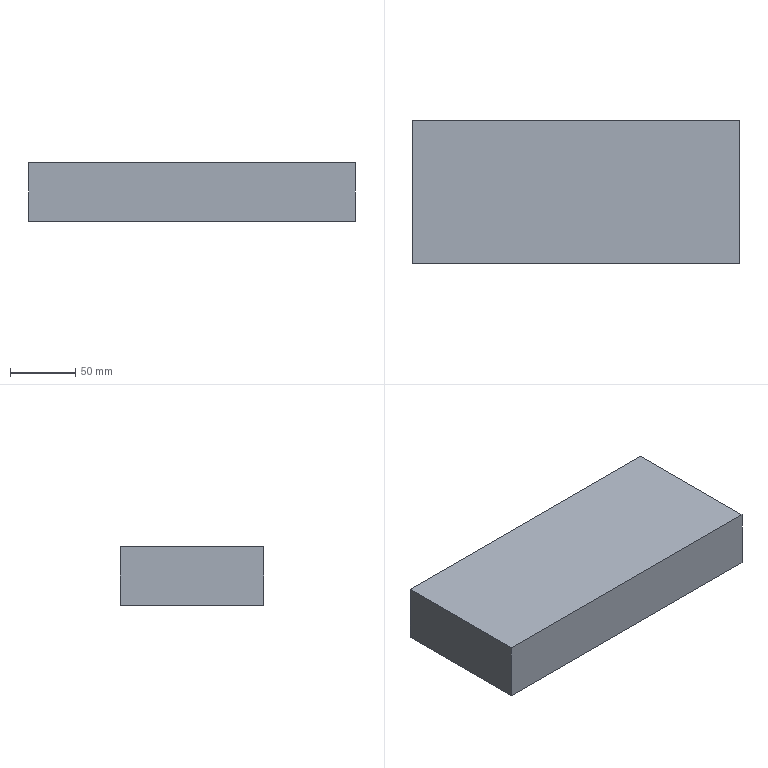Part | SolidWorks | features Extrusion 1 | 1 solid | 6 faces | box 250 x 110 x 45 mm | volume 1237500 mm3 | plane 6
STEP:
#1=CARTESIAN_POINT('',(-125.,55.,-22.5));
#2=VERTEX_POINT('',#1);
#3=CARTESIAN_POINT('',(-125.,-55.,-22.5));
#4=VERTEX_POINT('',#3);
#5=CARTESIAN_POINT('',(-125.,-55.,-22.5));
#6=DIRECTION('',(0.,-1.,0.));
#7=VECTOR('',#6,1000.);
#8=LINE('',#5,#7);
#9=EDGE_CURVE('',#2,#4,#8,.T.);
#10=ORIENTED_EDGE('',*,*,#9,.T.);
#11=CARTESIAN_POINT('',(-125.,-55.,22.5));
#12=VERTEX_POINT('',#11);
#13=CARTESIAN_POINT('',(-125.,-55.,22.5));
#14=DIRECTION('',(0.,0.,-1.));
#15=VECTOR('',#14,1000.);
#16=LINE('',#13,#15);
#17=EDGE_CURVE('',#12,#4,#16,.T.);
#18=ORIENTED_EDGE('',*,*,#17,.F.);
#19=CARTESIAN_POINT('',(-125.,55.,22.5));
#20=VERTEX_POINT('',#19);
#21=CARTESIAN_POINT('',(-125.,-55.,22.5));
#22=DIRECTION('',(0.,-1.,0.));
#23=VECTOR('',#22,1000.);
#24=LINE('',#21,#23);
#25=EDGE_CURVE('',#20,#12,#24,.T.);
#26=ORIENTED_EDGE('',*,*,#25,.F.);
#27=CARTESIAN_POINT('',(-125.,55.,22.5));
#28=DIRECTION('',(0.,0.,-1.));
#29=VECTOR('',#28,1000.);
#30=LINE('',#27,#29);
#31=EDGE_CURVE('',#20,#2,#30,.T.);
#32=ORIENTED_EDGE('',*,*,#31,.T.);
#33=EDGE_LOOP('',(#10,#18,#26,#32));
#34=FACE_OUTER_BOUND('',#33,.T.);
#35=CARTESIAN_POINT('',(-125.,-55.,22.5));
#36=DIRECTION('',(1.,0.,0.));
#37=DIRECTION('',(0.,0.,-1.));
#38=AXIS2_PLACEMENT_3D('',#35,#36,#37);
#39=PLANE('',#38);
#40=ADVANCED_FACE('',(#34),#39,.F.);
#41=CARTESIAN_POINT('',(125.,-55.,-22.5));
#42=VERTEX_POINT('',#41);
#43=CARTESIAN_POINT('',(125.,-55.,-22.5));
#44=DIRECTION('',(1.,0.,0.));
#45=VECTOR('',#44,1000.);
#46=LINE('',#43,#45);
#47=EDGE_CURVE('',#4,#42,#46,.T.);
#48=ORIENTED_EDGE('',*,*,#47,.T.);
#49=CARTESIAN_POINT('',(125.,-55.,22.5));
#50=VERTEX_POINT('',#49);
#51=CARTESIAN_POINT('',(125.,-55.,22.5));
#52=DIRECTION('',(0.,0.,-1.));
#53=VECTOR('',#52,1000.);
#54=LINE('',#51,#53);
#55=EDGE_CURVE('',#50,#42,#54,.T.);
#56=ORIENTED_EDGE('',*,*,#55,.F.);
#57=CARTESIAN_POINT('',(125.,-55.,22.5));
#58=DIRECTION('',(1.,0.,0.));
#59=VECTOR('',#58,1000.);
#60=LINE('',#57,#59);
#61=EDGE_CURVE('',#12,#50,#60,.T.);
#62=ORIENTED_EDGE('',*,*,#61,.F.);
#63=ORIENTED_EDGE('',*,*,#17,.T.);
#64=EDGE_LOOP('',(#48,#56,#62,#63));
#65=FACE_OUTER_BOUND('',#64,.T.);
#66=CARTESIAN_POINT('',(125.,-55.,22.5));
#67=DIRECTION('',(0.,1.,0.));
#68=DIRECTION('',(-1.,0.,0.));
#69=AXIS2_PLACEMENT_3D('',#66,#67,#68);
#70=PLANE('',#69);
#71=ADVANCED_FACE('',(#65),#70,.F.);
#72=CARTESIAN_POINT('',(125.,55.,-22.5));
#73=VERTEX_POINT('',#72);
#74=CARTESIAN_POINT('',(125.,-55.,-22.5));
#75=DIRECTION('',(0.,1.,0.));
#76=VECTOR('',#75,1000.);
#77=LINE('',#74,#76);
#78=EDGE_CURVE('',#42,#73,#77,.T.);
#79=ORIENTED_EDGE('',*,*,#78,.T.);
#80=CARTESIAN_POINT('',(125.,55.,22.5));
#81=VERTEX_POINT('',#80);
#82=CARTESIAN_POINT('',(125.,55.,22.5));
#83=DIRECTION('',(0.,0.,-1.));
#84=VECTOR('',#83,1000.);
#85=LINE('',#82,#84);
#86=EDGE_CURVE('',#81,#73,#85,.T.);
#87=ORIENTED_EDGE('',*,*,#86,.F.);
#88=CARTESIAN_POINT('',(125.,-55.,22.5));
#89=DIRECTION('',(0.,1.,0.));
#90=VECTOR('',#89,1000.);
#91=LINE('',#88,#90);
#92=EDGE_CURVE('',#50,#81,#91,.T.);
#93=ORIENTED_EDGE('',*,*,#92,.F.);
#94=ORIENTED_EDGE('',*,*,#55,.T.);
#95=EDGE_LOOP('',(#79,#87,#93,#94));
#96=FACE_OUTER_BOUND('',#95,.T.);
#97=CARTESIAN_POINT('',(125.,-55.,22.5));
#98=DIRECTION('',(-1.,0.,0.));
#99=DIRECTION('',(0.,0.,1.));
#100=AXIS2_PLACEMENT_3D('',#97,#98,#99);
#101=PLANE('',#100);
#102=ADVANCED_FACE('',(#96),#101,.F.);
#103=CARTESIAN_POINT('',(125.,55.,-22.5));
#104=DIRECTION('',(-1.,0.,0.));
#105=VECTOR('',#104,1000.);
#106=LINE('',#103,#105);
#107=EDGE_CURVE('',#73,#2,#106,.T.);
#108=ORIENTED_EDGE('',*,*,#107,.T.);
#109=ORIENTED_EDGE('',*,*,#31,.F.);
#110=CARTESIAN_POINT('',(125.,55.,22.5));
#111=DIRECTION('',(-1.,0.,0.));
#112=VECTOR('',#111,1000.);
#113=LINE('',#110,#112);
#114=EDGE_CURVE('',#81,#20,#113,.T.);
#115=ORIENTED_EDGE('',*,*,#114,.F.);
#116=ORIENTED_EDGE('',*,*,#86,.T.);
#117=EDGE_LOOP('',(#108,#109,#115,#116));
#118=FACE_OUTER_BOUND('',#117,.T.);
#119=CARTESIAN_POINT('',(125.,55.,22.5));
#120=DIRECTION('',(0.,-1.,0.));
#121=DIRECTION('',(1.,0.,0.));
#122=AXIS2_PLACEMENT_3D('',#119,#120,#121);
#123=PLANE('',#122);
#124=ADVANCED_FACE('',(#118),#123,.F.);
#125=ORIENTED_EDGE('',*,*,#25,.T.);
#126=ORIENTED_EDGE('',*,*,#61,.T.);
#127=ORIENTED_EDGE('',*,*,#92,.T.);
#128=ORIENTED_EDGE('',*,*,#114,.T.);
#129=EDGE_LOOP('',(#125,#126,#127,#128));
#130=FACE_OUTER_BOUND('',#129,.T.);
#131=CARTESIAN_POINT('',(0.,0.,22.5));
#132=DIRECTION('',(0.,0.,1.));
#133=DIRECTION('',(1.,0.,0.));
#134=AXIS2_PLACEMENT_3D('',#131,#132,#133);
#135=PLANE('',#134);
#136=ADVANCED_FACE('',(#130),#135,.T.);
#137=ORIENTED_EDGE('',*,*,#9,.F.);
#138=ORIENTED_EDGE('',*,*,#107,.F.);
#139=ORIENTED_EDGE('',*,*,#78,.F.);
#140=ORIENTED_EDGE('',*,*,#47,.F.);
#141=EDGE_LOOP('',(#137,#138,#139,#140));
#142=FACE_OUTER_BOUND('',#141,.T.);
#143=CARTESIAN_POINT('',(0.,0.,-22.5));
#144=DIRECTION('',(0.,0.,1.));
#145=DIRECTION('',(1.,0.,0.));
#146=AXIS2_PLACEMENT_3D('',#143,#144,#145);
#147=PLANE('',#146);
#148=ADVANCED_FACE('',(#142),#147,.F.);
#149=CLOSED_SHELL('',(#40,#71,#102,#124,#136,#148));
#150=MANIFOLD_SOLID_BREP('',#149);
#151=CARTESIAN_POINT('',(0.,0.,0.));
#152=DIRECTION('',(0.,0.,1.));
#153=DIRECTION('',(1.,0.,0.));
#154=AXIS2_PLACEMENT_3D('',#151,#152,#153);
#155=(LENGTH_UNIT()NAMED_UNIT(*)SI_UNIT(.MILLI.,.METRE.));
#156=UNCERTAINTY_MEASURE_WITH_UNIT(LENGTH_MEASURE(0.00001),#155,'','');
#157=(NAMED_UNIT(*)PLANE_ANGLE_UNIT()SI_UNIT($,.RADIAN.));
#158=(NAMED_UNIT(*)SI_UNIT($,.STERADIAN.)SOLID_ANGLE_UNIT());
#159=(GEOMETRIC_REPRESENTATION_CONTEXT(3)GLOBAL_UNCERTAINTY_ASSIGNED_CONTEXT((#156))GLOBAL_UNIT_ASSIGNED_CONTEXT((#155,#157,#158))REPRESENTATION_CONTEXT('',''));
#160=ADVANCED_BREP_SHAPE_REPRESENTATION('',(#150,#154),#159);